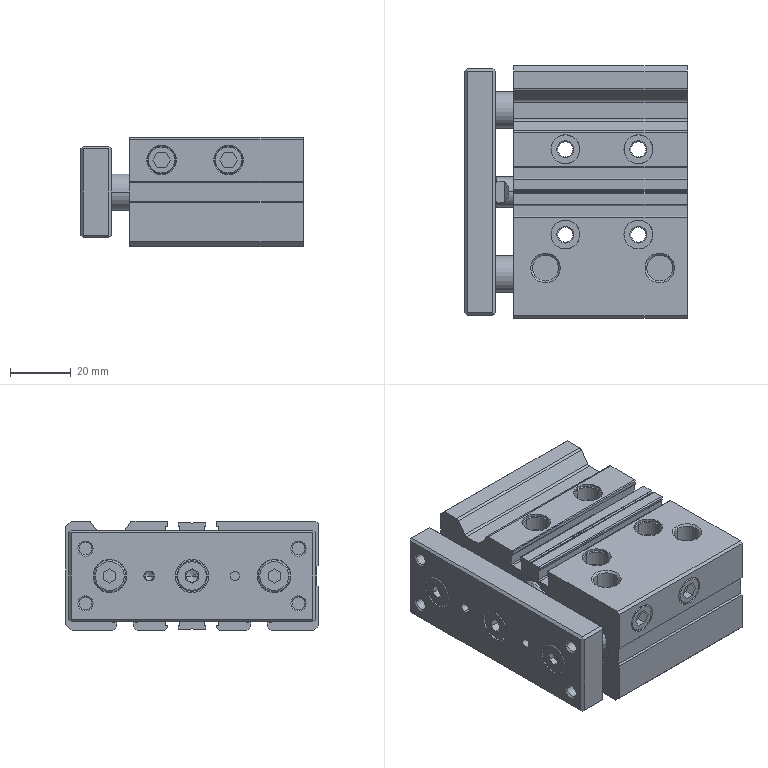Part | STEP file | Three-axis cylinder TCM-20x20-S | 4 solids | 561 faces | box 73 x 83 x 36 mm | volume 154063 mm3 | cylinder 231 | plane 210 | cone 102 | torus 18 | commonest cylinder face diameters 3 x21 0.8 x20 0.4 x18 4.134 x16 9.5 x16 1.8 x12